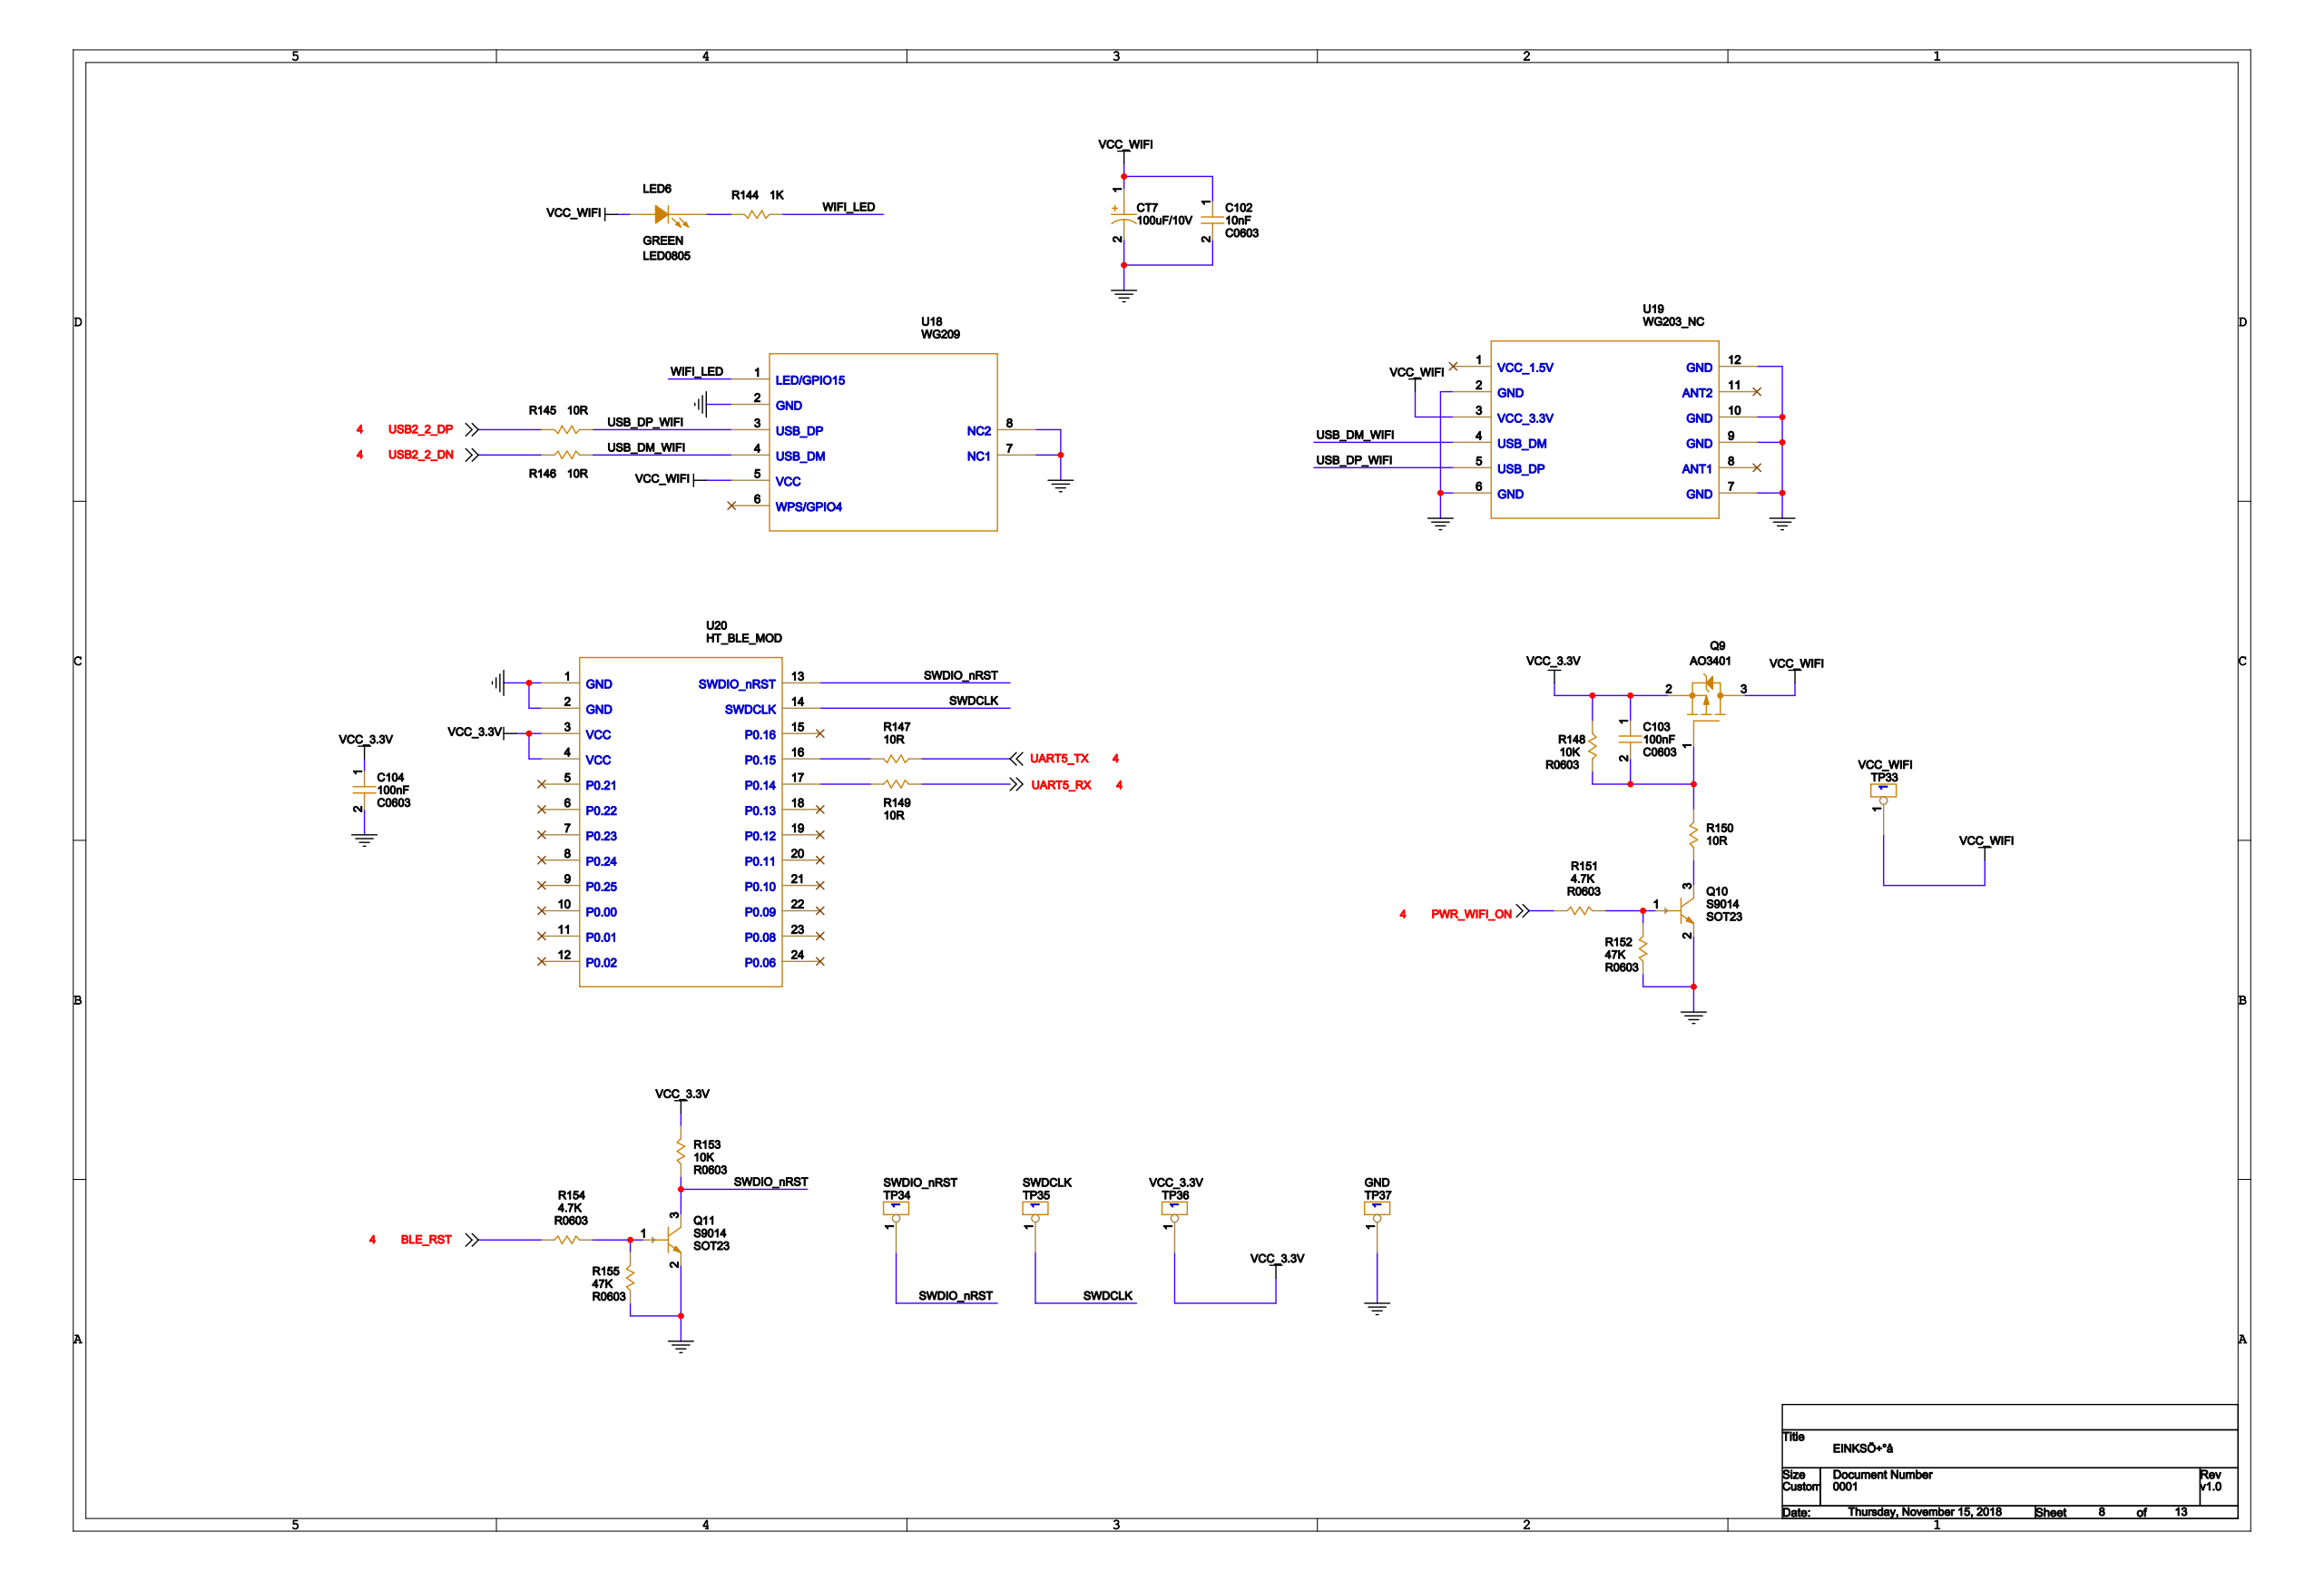Circuit board | Cadence Allegro | 609 parts | 409 nets | one sheet of the schematic
Parts on this sheet (reference | value | footprint):
C102 | 10nF | C0603
C103 | 100nF | C0603
C104 | 100nF | C0603
CT7 | 100uF/10V | B_CASE
LED6 | GREEN | LED0805
Q9 | AO3401 | SOT23
Q10 | S9014 | SOT23
Q11 | S9014 | SOT23
R144 | 1K | R0603
R145 | 10R | R0603
R146 | 10R | R0603
R147 | 10R | R0603
R148 | 10K | R0603
R149 | 10R | R0603
R150 | 10R | R0603
R151 | 4.7K | R0603
R152 | 47K | R0603
R153 | 10K | R0603
R154 | 4.7K | R0603
R155 | 47K | R0603
TP33 | VCC_WIFI | TP_50
TP34 | SWDIO_nRST | TP_50
TP35 | SWDCLK | TP_50
TP36 | VCC_3.3V | TP_50
TP37 | GND | TP_50
U18 | WG209 | WG209_SMD
U19 | WG203_NC | WG203
U20 | HT_BLE_MOD | HT_BLE_MOD_A2
Nets of these parts (net: part-pin ...):
GND: C102-2 C104-2 CT7-2 Q10-2 Q11-2 R152-2 R155-2 TP37-1 U18-2 U18-7 U18-8 U19-2 U19-6 U19-7 U19-9 U19-10 U19-12 U20-1 U20-2
VCC_3.3V: C103-1 C104-1 Q9-2 R148-2 R153-2 TP36-1 U20-3 U20-4
VCC_WIFI: C102-1 CT7-1 LED6-2 Q9-3 TP33-1 U18-5 U19-3
PWR_WIFI_ON: R151-2
BLE_RST: R154-2
UART5_RX: R149-1
UART5_TX: R147-1
USB2_2_DN: R146-2
USB2_2_DP: R145-2
N27836578: LED6-1 R144-2
N28129642: C103-2 Q9-1 R148-1 R150-1
N28129596: Q10-1 R151-1 R152-1
N27836597: Q11-1 R154-1 R155-1
WIFI_LED: R144-1 U18-1
USB_DM_WIFI: R146-1 U18-4 U19-4
N27836590: R147-2 U20-16
N27836591: R149-2 U20-17
USB_DP_WIFI: R145-1 U18-3 U19-5
N28129660: Q10-3 R150-2
SWDIO_NRST: Q11-3 R153-1 TP34-1 U20-13
SWDCLK: TP35-1 U20-14